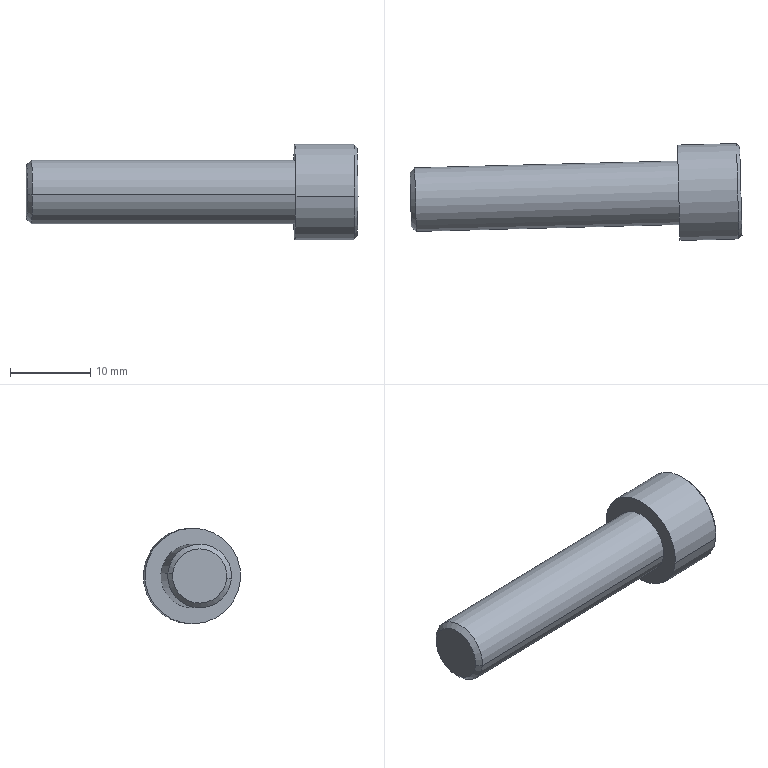Part | STEP file | 1_id1282_x_t | 1 solid | 20 faces | box 41.278 x 12.093 x 11.906 mm | volume 2345 mm3 | plane 10 | cone 6 | cylinder 4 | commonest cylinder face diameters 7.938 x2 11.906 x2